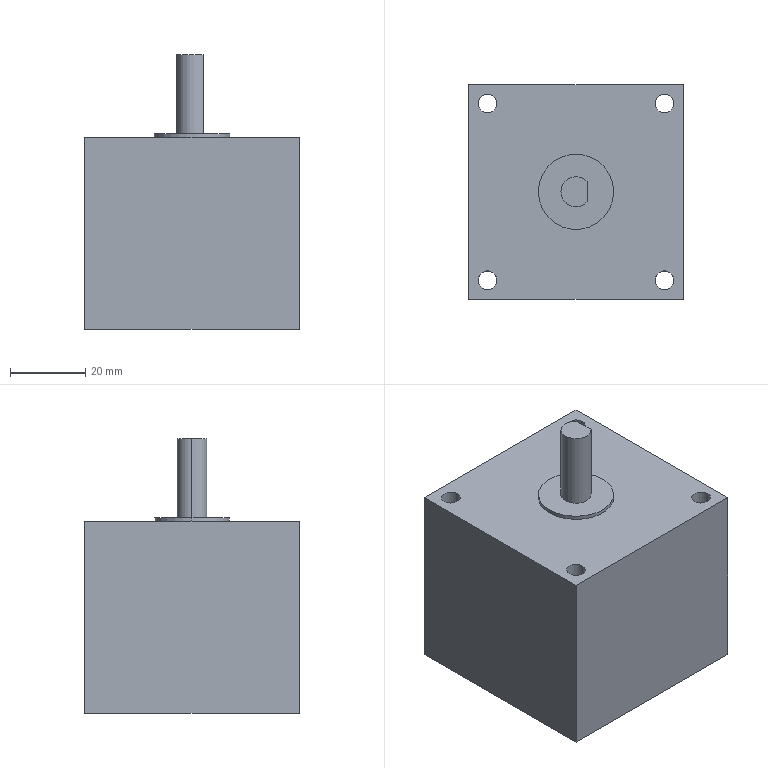Part | SolidWorks | features ICE 4, Extrusion 1 | 1 solid | 21 faces | box 57 x 57 x 73 mm | volume 162987 mm3 | cylinder 12 | plane 9 | commonest cylinder face diameters 5 x8 8 x2 20 x2
STEP:
#1=CARTESIAN_POINT('',(-4.,0.,73.));
#2=VERTEX_POINT('',#1);
#3=CARTESIAN_POINT('',(3.,-2.646,73.));
#4=VERTEX_POINT('',#3);
#5=CARTESIAN_POINT('',(0.,0.,73.));
#6=DIRECTION('',(0.,0.,1.));
#7=DIRECTION('',(1.,0.,0.));
#8=AXIS2_PLACEMENT_3D('',#5,#6,#7);
#9=CIRCLE('',#8,4.);
#10=EDGE_CURVE('',#2,#4,#9,.T.);
#11=ORIENTED_EDGE('',*,*,#10,.F.);
#12=CARTESIAN_POINT('',(-4.,0.,52.));
#13=VERTEX_POINT('',#12);
#14=CARTESIAN_POINT('',(-4.,0.,73.));
#15=DIRECTION('',(0.,0.,-1.));
#16=VECTOR('',#15,1000.);
#17=LINE('',#14,#16);
#18=EDGE_CURVE('',#2,#13,#17,.T.);
#19=ORIENTED_EDGE('',*,*,#18,.T.);
#20=CARTESIAN_POINT('',(3.,-2.646,52.));
#21=VERTEX_POINT('',#20);
#22=CARTESIAN_POINT('',(0.,0.,52.));
#23=DIRECTION('',(0.,0.,1.));
#24=DIRECTION('',(1.,0.,0.));
#25=AXIS2_PLACEMENT_3D('',#22,#23,#24);
#26=CIRCLE('',#25,4.);
#27=EDGE_CURVE('',#13,#21,#26,.T.);
#28=ORIENTED_EDGE('',*,*,#27,.T.);
#29=CARTESIAN_POINT('',(3.,-2.646,52.));
#30=DIRECTION('',(0.,0.,1.));
#31=VECTOR('',#30,1000.);
#32=LINE('',#29,#31);
#33=EDGE_CURVE('',#21,#4,#32,.T.);
#34=ORIENTED_EDGE('',*,*,#33,.T.);
#35=EDGE_LOOP('',(#11,#19,#28,#34));
#36=FACE_OUTER_BOUND('',#35,.T.);
#37=CARTESIAN_POINT('',(0.,0.,73.));
#38=DIRECTION('',(0.,0.,-1.));
#39=DIRECTION('',(-1.,0.,0.));
#40=AXIS2_PLACEMENT_3D('',#37,#38,#39);
#41=CYLINDRICAL_SURFACE('',#40,4.);
#42=ADVANCED_FACE('',(#36),#41,.T.);
#43=CARTESIAN_POINT('',(10.,0.,52.));
#44=VERTEX_POINT('',#43);
#45=CARTESIAN_POINT('',(-10.,0.,52.));
#46=VERTEX_POINT('',#45);
#47=CARTESIAN_POINT('',(0.,0.,52.));
#48=DIRECTION('',(0.,0.,1.));
#49=DIRECTION('',(1.,0.,0.));
#50=AXIS2_PLACEMENT_3D('',#47,#48,#49);
#51=CIRCLE('',#50,10.);
#52=EDGE_CURVE('',#44,#46,#51,.T.);
#53=ORIENTED_EDGE('',*,*,#52,.F.);
#54=CARTESIAN_POINT('',(10.,0.,51.));
#55=VERTEX_POINT('',#54);
#56=CARTESIAN_POINT('',(10.,0.,52.));
#57=DIRECTION('',(0.,0.,-1.));
#58=VECTOR('',#57,1000.);
#59=LINE('',#56,#58);
#60=EDGE_CURVE('',#44,#55,#59,.T.);
#61=ORIENTED_EDGE('',*,*,#60,.T.);
#62=CARTESIAN_POINT('',(-10.,0.,51.));
#63=VERTEX_POINT('',#62);
#64=CARTESIAN_POINT('',(0.,0.,51.));
#65=DIRECTION('',(0.,0.,1.));
#66=DIRECTION('',(1.,0.,0.));
#67=AXIS2_PLACEMENT_3D('',#64,#65,#66);
#68=CIRCLE('',#67,10.);
#69=EDGE_CURVE('',#55,#63,#68,.T.);
#70=ORIENTED_EDGE('',*,*,#69,.T.);
#71=CARTESIAN_POINT('',(-10.,0.,52.));
#72=DIRECTION('',(0.,0.,-1.));
#73=VECTOR('',#72,1000.);
#74=LINE('',#71,#73);
#75=EDGE_CURVE('',#46,#63,#74,.T.);
#76=ORIENTED_EDGE('',*,*,#75,.F.);
#77=EDGE_LOOP('',(#53,#61,#70,#76));
#78=FACE_OUTER_BOUND('',#77,.T.);
#79=CARTESIAN_POINT('',(0.,0.,52.));
#80=DIRECTION('',(0.,0.,-1.));
#81=DIRECTION('',(-1.,0.,0.));
#82=AXIS2_PLACEMENT_3D('',#79,#80,#81);
#83=CYLINDRICAL_SURFACE('',#82,10.);
#84=ADVANCED_FACE('',(#78),#83,.T.);
#85=CARTESIAN_POINT('',(-26.,-23.5,0.));
#86=VERTEX_POINT('',#85);
#87=CARTESIAN_POINT('',(-21.,-23.5,0.));
#88=VERTEX_POINT('',#87);
#89=CARTESIAN_POINT('',(-23.5,-23.5,0.));
#90=DIRECTION('',(0.,0.,1.));
#91=DIRECTION('',(1.,0.,0.));
#92=AXIS2_PLACEMENT_3D('',#89,#90,#91);
#93=CIRCLE('',#92,2.5);
#94=EDGE_CURVE('',#86,#88,#93,.T.);
#95=ORIENTED_EDGE('',*,*,#94,.F.);
#96=CARTESIAN_POINT('',(-26.,-23.5,51.));
#97=VERTEX_POINT('',#96);
#98=CARTESIAN_POINT('',(-26.,-23.5,-47.));
#99=DIRECTION('',(0.,0.,1.));
#100=VECTOR('',#99,1000.);
#101=LINE('',#98,#100);
#102=EDGE_CURVE('',#86,#97,#101,.T.);
#103=ORIENTED_EDGE('',*,*,#102,.T.);
#104=CARTESIAN_POINT('',(-21.,-23.5,51.));
#105=VERTEX_POINT('',#104);
#106=CARTESIAN_POINT('',(-23.5,-23.5,51.));
#107=DIRECTION('',(0.,0.,1.));
#108=DIRECTION('',(1.,0.,0.));
#109=AXIS2_PLACEMENT_3D('',#106,#107,#108);
#110=CIRCLE('',#109,2.5);
#111=EDGE_CURVE('',#97,#105,#110,.T.);
#112=ORIENTED_EDGE('',*,*,#111,.T.);
#113=CARTESIAN_POINT('',(-21.,-23.5,-47.));
#114=DIRECTION('',(0.,0.,1.));
#115=VECTOR('',#114,1000.);
#116=LINE('',#113,#115);
#117=EDGE_CURVE('',#88,#105,#116,.T.);
#118=ORIENTED_EDGE('',*,*,#117,.F.);
#119=EDGE_LOOP('',(#95,#103,#112,#118));
#120=FACE_OUTER_BOUND('',#119,.T.);
#121=CARTESIAN_POINT('',(-23.5,-23.5,-47.));
#122=DIRECTION('',(0.,0.,1.));
#123=DIRECTION('',(1.,0.,0.));
#124=AXIS2_PLACEMENT_3D('',#121,#122,#123);
#125=CYLINDRICAL_SURFACE('',#124,2.5);
#126=ADVANCED_FACE('',(#120),#125,.F.);
#127=CARTESIAN_POINT('',(21.,-23.5,0.));
#128=VERTEX_POINT('',#127);
#129=CARTESIAN_POINT('',(26.,-23.5,0.));
#130=VERTEX_POINT('',#129);
#131=CARTESIAN_POINT('',(23.5,-23.5,0.));
#132=DIRECTION('',(0.,0.,1.));
#133=DIRECTION('',(1.,0.,0.));
#134=AXIS2_PLACEMENT_3D('',#131,#132,#133);
#135=CIRCLE('',#134,2.5);
#136=EDGE_CURVE('',#128,#130,#135,.T.);
#137=ORIENTED_EDGE('',*,*,#136,.F.);
#138=CARTESIAN_POINT('',(21.,-23.5,51.));
#139=VERTEX_POINT('',#138);
#140=CARTESIAN_POINT('',(21.,-23.5,-47.));
#141=DIRECTION('',(0.,0.,1.));
#142=VECTOR('',#141,1000.);
#143=LINE('',#140,#142);
#144=EDGE_CURVE('',#128,#139,#143,.T.);
#145=ORIENTED_EDGE('',*,*,#144,.T.);
#146=CARTESIAN_POINT('',(26.,-23.5,51.));
#147=VERTEX_POINT('',#146);
#148=CARTESIAN_POINT('',(23.5,-23.5,51.));
#149=DIRECTION('',(0.,0.,1.));
#150=DIRECTION('',(1.,0.,0.));
#151=AXIS2_PLACEMENT_3D('',#148,#149,#150);
#152=CIRCLE('',#151,2.5);
#153=EDGE_CURVE('',#139,#147,#152,.T.);
#154=ORIENTED_EDGE('',*,*,#153,.T.);
#155=CARTESIAN_POINT('',(26.,-23.5,-47.));
#156=DIRECTION('',(0.,0.,1.));
#157=VECTOR('',#156,1000.);
#158=LINE('',#155,#157);
#159=EDGE_CURVE('',#130,#147,#158,.T.);
#160=ORIENTED_EDGE('',*,*,#159,.F.);
#161=EDGE_LOOP('',(#137,#145,#154,#160));
#162=FACE_OUTER_BOUND('',#161,.T.);
#163=CARTESIAN_POINT('',(23.5,-23.5,-47.));
#164=DIRECTION('',(0.,0.,1.));
#165=DIRECTION('',(1.,0.,0.));
#166=AXIS2_PLACEMENT_3D('',#163,#164,#165);
#167=CYLINDRICAL_SURFACE('',#166,2.5);
#168=ADVANCED_FACE('',(#162),#167,.F.);
#169=CARTESIAN_POINT('',(21.,23.5,0.));
#170=VERTEX_POINT('',#169);
#171=CARTESIAN_POINT('',(26.,23.5,0.));
#172=VERTEX_POINT('',#171);
#173=CARTESIAN_POINT('',(23.5,23.5,0.));
#174=DIRECTION('',(0.,0.,1.));
#175=DIRECTION('',(1.,0.,0.));
#176=AXIS2_PLACEMENT_3D('',#173,#174,#175);
#177=CIRCLE('',#176,2.5);
#178=EDGE_CURVE('',#170,#172,#177,.T.);
#179=ORIENTED_EDGE('',*,*,#178,.F.);
#180=CARTESIAN_POINT('',(21.,23.5,51.));
#181=VERTEX_POINT('',#180);
#182=CARTESIAN_POINT('',(21.,23.5,-47.));
#183=DIRECTION('',(0.,0.,1.));
#184=VECTOR('',#183,1000.);
#185=LINE('',#182,#184);
#186=EDGE_CURVE('',#170,#181,#185,.T.);
#187=ORIENTED_EDGE('',*,*,#186,.T.);
#188=CARTESIAN_POINT('',(26.,23.5,51.));
#189=VERTEX_POINT('',#188);
#190=CARTESIAN_POINT('',(23.5,23.5,51.));
#191=DIRECTION('',(0.,0.,1.));
#192=DIRECTION('',(1.,0.,0.));
#193=AXIS2_PLACEMENT_3D('',#190,#191,#192);
#194=CIRCLE('',#193,2.5);
#195=EDGE_CURVE('',#181,#189,#194,.T.);
#196=ORIENTED_EDGE('',*,*,#195,.T.);
#197=CARTESIAN_POINT('',(26.,23.5,-47.));
#198=DIRECTION('',(0.,0.,1.));
#199=VECTOR('',#198,1000.);
#200=LINE('',#197,#199);
#201=EDGE_CURVE('',#172,#189,#200,.T.);
#202=ORIENTED_EDGE('',*,*,#201,.F.);
#203=EDGE_LOOP('',(#179,#187,#196,#202));
#204=FACE_OUTER_BOUND('',#203,.T.);
#205=CARTESIAN_POINT('',(23.5,23.5,-47.));
#206=DIRECTION('',(0.,0.,1.));
#207=DIRECTION('',(1.,0.,0.));
#208=AXIS2_PLACEMENT_3D('',#205,#206,#207);
#209=CYLINDRICAL_SURFACE('',#208,2.5);
#210=ADVANCED_FACE('',(#204),#209,.F.);
#211=CARTESIAN_POINT('',(-26.,23.5,0.));
#212=VERTEX_POINT('',#211);
#213=CARTESIAN_POINT('',(-21.,23.5,0.));
#214=VERTEX_POINT('',#213);
#215=CARTESIAN_POINT('',(-23.5,23.5,0.));
#216=DIRECTION('',(0.,0.,1.));
#217=DIRECTION('',(1.,0.,0.));
#218=AXIS2_PLACEMENT_3D('',#215,#216,#217);
#219=CIRCLE('',#218,2.5);
#220=EDGE_CURVE('',#212,#214,#219,.T.);
#221=ORIENTED_EDGE('',*,*,#220,.F.);
#222=CARTESIAN_POINT('',(-26.,23.5,51.));
#223=VERTEX_POINT('',#222);
#224=CARTESIAN_POINT('',(-26.,23.5,-47.));
#225=DIRECTION('',(0.,0.,1.));
#226=VECTOR('',#225,1000.);
#227=LINE('',#224,#226);
#228=EDGE_CURVE('',#212,#223,#227,.T.);
#229=ORIENTED_EDGE('',*,*,#228,.T.);
#230=CARTESIAN_POINT('',(-21.,23.5,51.));
#231=VERTEX_POINT('',#230);
#232=CARTESIAN_POINT('',(-23.5,23.5,51.));
#233=DIRECTION('',(0.,0.,1.));
#234=DIRECTION('',(1.,0.,0.));
#235=AXIS2_PLACEMENT_3D('',#232,#233,#234);
#236=CIRCLE('',#235,2.5);
#237=EDGE_CURVE('',#223,#231,#236,.T.);
#238=ORIENTED_EDGE('',*,*,#237,.T.);
#239=CARTESIAN_POINT('',(-21.,23.5,-47.));
#240=DIRECTION('',(0.,0.,1.));
#241=VECTOR('',#240,1000.);
#242=LINE('',#239,#241);
#243=EDGE_CURVE('',#214,#231,#242,.T.);
#244=ORIENTED_EDGE('',*,*,#243,.F.);
#245=EDGE_LOOP('',(#221,#229,#238,#244));
#246=FACE_OUTER_BOUND('',#245,.T.);
#247=CARTESIAN_POINT('',(-23.5,23.5,-47.));
#248=DIRECTION('',(0.,0.,1.));
#249=DIRECTION('',(1.,0.,0.));
#250=AXIS2_PLACEMENT_3D('',#247,#248,#249);
#251=CYLINDRICAL_SURFACE('',#250,2.5);
#252=ADVANCED_FACE('',(#246),#251,.F.);
#253=CARTESIAN_POINT('',(-28.5,28.5,0.));
#254=VERTEX_POINT('',#253);
#255=CARTESIAN_POINT('',(-28.5,-28.5,0.));
#256=VERTEX_POINT('',#255);
#257=CARTESIAN_POINT('',(-28.5,-28.5,0.));
#258=DIRECTION('',(0.,-1.,0.));
#259=VECTOR('',#258,1000.);
#260=LINE('',#257,#259);
#261=EDGE_CURVE('',#254,#256,#260,.T.);
#262=ORIENTED_EDGE('',*,*,#261,.T.);
#263=CARTESIAN_POINT('',(-28.5,-28.5,51.));
#264=VERTEX_POINT('',#263);
#265=CARTESIAN_POINT('',(-28.5,-28.5,51.));
#266=DIRECTION('',(0.,0.,-1.));
#267=VECTOR('',#266,1000.);
#268=LINE('',#265,#267);
#269=EDGE_CURVE('',#264,#256,#268,.T.);
#270=ORIENTED_EDGE('',*,*,#269,.F.);
#271=CARTESIAN_POINT('',(-28.5,28.5,51.));
#272=VERTEX_POINT('',#271);
#273=CARTESIAN_POINT('',(-28.5,-28.5,51.));
#274=DIRECTION('',(0.,-1.,0.));
#275=VECTOR('',#274,1000.);
#276=LINE('',#273,#275);
#277=EDGE_CURVE('',#272,#264,#276,.T.);
#278=ORIENTED_EDGE('',*,*,#277,.F.);
#279=CARTESIAN_POINT('',(-28.5,28.5,51.));
#280=DIRECTION('',(0.,0.,-1.));
#281=VECTOR('',#280,1000.);
#282=LINE('',#279,#281);
#283=EDGE_CURVE('',#272,#254,#282,.T.);
#284=ORIENTED_EDGE('',*,*,#283,.T.);
#285=EDGE_LOOP('',(#262,#270,#278,#284));
#286=FACE_OUTER_BOUND('',#285,.T.);
#287=CARTESIAN_POINT('',(-28.5,-28.5,51.));
#288=DIRECTION('',(1.,0.,0.));
#289=DIRECTION('',(0.,0.,-1.));
#290=AXIS2_PLACEMENT_3D('',#287,#288,#289);
#291=PLANE('',#290);
#292=ADVANCED_FACE('',(#286),#291,.F.);
#293=CARTESIAN_POINT('',(28.5,-28.5,0.));
#294=VERTEX_POINT('',#293);
#295=CARTESIAN_POINT('',(28.5,-28.5,0.));
#296=DIRECTION('',(1.,0.,0.));
#297=VECTOR('',#296,1000.);
#298=LINE('',#295,#297);
#299=EDGE_CURVE('',#256,#294,#298,.T.);
#300=ORIENTED_EDGE('',*,*,#299,.T.);
#301=CARTESIAN_POINT('',(28.5,-28.5,51.));
#302=VERTEX_POINT('',#301);
#303=CARTESIAN_POINT('',(28.5,-28.5,51.));
#304=DIRECTION('',(0.,0.,-1.));
#305=VECTOR('',#304,1000.);
#306=LINE('',#303,#305);
#307=EDGE_CURVE('',#302,#294,#306,.T.);
#308=ORIENTED_EDGE('',*,*,#307,.F.);
#309=CARTESIAN_POINT('',(28.5,-28.5,51.));
#310=DIRECTION('',(1.,0.,0.));
#311=VECTOR('',#310,1000.);
#312=LINE('',#309,#311);
#313=EDGE_CURVE('',#264,#302,#312,.T.);
#314=ORIENTED_EDGE('',*,*,#313,.F.);
#315=ORIENTED_EDGE('',*,*,#269,.T.);
#316=EDGE_LOOP('',(#300,#308,#314,#315));
#317=FACE_OUTER_BOUND('',#316,.T.);
#318=CARTESIAN_POINT('',(28.5,-28.5,51.));
#319=DIRECTION('',(0.,1.,0.));
#320=DIRECTION('',(-1.,0.,0.));
#321=AXIS2_PLACEMENT_3D('',#318,#319,#320);
#322=PLANE('',#321);
#323=ADVANCED_FACE('',(#317),#322,.F.);
#324=CARTESIAN_POINT('',(28.5,28.5,0.));
#325=VERTEX_POINT('',#324);
#326=CARTESIAN_POINT('',(28.5,-28.5,0.));
#327=DIRECTION('',(0.,1.,0.));
#328=VECTOR('',#327,1000.);
#329=LINE('',#326,#328);
#330=EDGE_CURVE('',#294,#325,#329,.T.);
#331=ORIENTED_EDGE('',*,*,#330,.T.);
#332=CARTESIAN_POINT('',(28.5,28.5,51.));
#333=VERTEX_POINT('',#332);
#334=CARTESIAN_POINT('',(28.5,28.5,51.));
#335=DIRECTION('',(0.,0.,-1.));
#336=VECTOR('',#335,1000.);
#337=LINE('',#334,#336);
#338=EDGE_CURVE('',#333,#325,#337,.T.);
#339=ORIENTED_EDGE('',*,*,#338,.F.);
#340=CARTESIAN_POINT('',(28.5,-28.5,51.));
#341=DIRECTION('',(0.,1.,0.));
#342=VECTOR('',#341,1000.);
#343=LINE('',#340,#342);
#344=EDGE_CURVE('',#302,#333,#343,.T.);
#345=ORIENTED_EDGE('',*,*,#344,.F.);
#346=ORIENTED_EDGE('',*,*,#307,.T.);
#347=EDGE_LOOP('',(#331,#339,#345,#346));
#348=FACE_OUTER_BOUND('',#347,.T.);
#349=CARTESIAN_POINT('',(28.5,-28.5,51.));
#350=DIRECTION('',(-1.,0.,0.));
#351=DIRECTION('',(0.,0.,1.));
#352=AXIS2_PLACEMENT_3D('',#349,#350,#351);
#353=PLANE('',#352);
#354=ADVANCED_FACE('',(#348),#353,.F.);
#355=CARTESIAN_POINT('',(28.5,28.5,0.));
#356=DIRECTION('',(-1.,0.,0.));
#357=VECTOR('',#356,1000.);
#358=LINE('',#355,#357);
#359=EDGE_CURVE('',#325,#254,#358,.T.);
#360=ORIENTED_EDGE('',*,*,#359,.T.);
#361=ORIENTED_EDGE('',*,*,#283,.F.);
#362=CARTESIAN_POINT('',(28.5,28.5,51.));
#363=DIRECTION('',(-1.,0.,0.));
#364=VECTOR('',#363,1000.);
#365=LINE('',#362,#364);
#366=EDGE_CURVE('',#333,#272,#365,.T.);
#367=ORIENTED_EDGE('',*,*,#366,.F.);
#368=ORIENTED_EDGE('',*,*,#338,.T.);
#369=EDGE_LOOP('',(#360,#361,#367,#368));
#370=FACE_OUTER_BOUND('',#369,.T.);
#371=CARTESIAN_POINT('',(28.5,28.5,51.));
#372=DIRECTION('',(0.,-1.,0.));
#373=DIRECTION('',(1.,0.,0.));
#374=AXIS2_PLACEMENT_3D('',#371,#372,#373);
#375=PLANE('',#374);
#376=ADVANCED_FACE('',(#370),#375,.F.);
#377=CARTESIAN_POINT('',(0.,0.,51.));
#378=DIRECTION('',(0.,0.,1.));
#379=DIRECTION('',(1.,0.,0.));
#380=AXIS2_PLACEMENT_3D('',#377,#378,#379);
#381=CIRCLE('',#380,10.);
#382=EDGE_CURVE('',#63,#55,#381,.T.);
#383=ORIENTED_EDGE('',*,*,#382,.F.);
#384=ORIENTED_EDGE('',*,*,#69,.F.);
#385=EDGE_LOOP('',(#383,#384));
#386=FACE_BOUND('',#385,.T.);
#387=CARTESIAN_POINT('',(-23.5,-23.5,51.));
#388=DIRECTION('',(0.,0.,1.));
#389=DIRECTION('',(1.,0.,0.));
#390=AXIS2_PLACEMENT_3D('',#387,#388,#389);
#391=CIRCLE('',#390,2.5);
#392=EDGE_CURVE('',#105,#97,#391,.T.);
#393=ORIENTED_EDGE('',*,*,#392,.F.);
#394=ORIENTED_EDGE('',*,*,#111,.F.);
#395=EDGE_LOOP('',(#393,#394));
#396=FACE_BOUND('',#395,.T.);
#397=CARTESIAN_POINT('',(23.5,-23.5,51.));
#398=DIRECTION('',(0.,0.,1.));
#399=DIRECTION('',(1.,0.,0.));
#400=AXIS2_PLACEMENT_3D('',#397,#398,#399);
#401=CIRCLE('',#400,2.5);
#402=EDGE_CURVE('',#147,#139,#401,.T.);
#403=ORIENTED_EDGE('',*,*,#402,.F.);
#404=ORIENTED_EDGE('',*,*,#153,.F.);
#405=EDGE_LOOP('',(#403,#404));
#406=FACE_BOUND('',#405,.T.);
#407=CARTESIAN_POINT('',(23.5,23.5,51.));
#408=DIRECTION('',(0.,0.,1.));
#409=DIRECTION('',(1.,0.,0.));
#410=AXIS2_PLACEMENT_3D('',#407,#408,#409);
#411=CIRCLE('',#410,2.5);
#412=EDGE_CURVE('',#189,#181,#411,.T.);
#413=ORIENTED_EDGE('',*,*,#412,.F.);
#414=ORIENTED_EDGE('',*,*,#195,.F.);
#415=EDGE_LOOP('',(#413,#414));
#416=FACE_BOUND('',#415,.T.);
#417=CARTESIAN_POINT('',(-23.5,23.5,51.));
#418=DIRECTION('',(0.,0.,1.));
#419=DIRECTION('',(1.,0.,0.));
#420=AXIS2_PLACEMENT_3D('',#417,#418,#419);
#421=CIRCLE('',#420,2.5);
#422=EDGE_CURVE('',#231,#223,#421,.T.);
#423=ORIENTED_EDGE('',*,*,#422,.F.);
#424=ORIENTED_EDGE('',*,*,#237,.F.);
#425=EDGE_LOOP('',(#423,#424));
#426=FACE_BOUND('',#425,.T.);
#427=ORIENTED_EDGE('',*,*,#277,.T.);
#428=ORIENTED_EDGE('',*,*,#313,.T.);
#429=ORIENTED_EDGE('',*,*,#344,.T.);
#430=ORIENTED_EDGE('',*,*,#366,.T.);
#431=EDGE_LOOP('',(#427,#428,#429,#430));
#432=FACE_OUTER_BOUND('',#431,.T.);
#433=CARTESIAN_POINT('',(0.,0.,51.));
#434=DIRECTION('',(0.,0.,1.));
#435=DIRECTION('',(1.,0.,0.));
#436=AXIS2_PLACEMENT_3D('',#433,#434,#435);
#437=PLANE('',#436);
#438=ADVANCED_FACE('',(#386,#396,#406,#416,#426,#432),#437,.T.);
#439=CARTESIAN_POINT('',(-23.5,-23.5,0.));
#440=DIRECTION('',(0.,0.,1.));
#441=DIRECTION('',(1.,0.,0.));
#442=AXIS2_PLACEMENT_3D('',#439,#440,#441);
#443=CIRCLE('',#442,2.5);
#444=EDGE_CURVE('',#88,#86,#443,.T.);
#445=ORIENTED_EDGE('',*,*,#444,.T.);
#446=ORIENTED_EDGE('',*,*,#94,.T.);
#447=EDGE_LOOP('',(#445,#446));
#448=FACE_BOUND('',#447,.T.);
#449=CARTESIAN_POINT('',(23.5,-23.5,0.));
#450=DIRECTION('',(0.,0.,1.));
#451=DIRECTION('',(1.,0.,0.));
#452=AXIS2_PLACEMENT_3D('',#449,#450,#451);
#453=CIRCLE('',#452,2.5);
#454=EDGE_CURVE('',#130,#128,#453,.T.);
#455=ORIENTED_EDGE('',*,*,#454,.T.);
#456=ORIENTED_EDGE('',*,*,#136,.T.);
#457=EDGE_LOOP('',(#455,#456));
#458=FACE_BOUND('',#457,.T.);
#459=CARTESIAN_POINT('',(23.5,23.5,0.));
#460=DIRECTION('',(0.,0.,1.));
#461=DIRECTION('',(1.,0.,0.));
#462=AXIS2_PLACEMENT_3D('',#459,#460,#461);
#463=CIRCLE('',#462,2.5);
#464=EDGE_CURVE('',#172,#170,#463,.T.);
#465=ORIENTED_EDGE('',*,*,#464,.T.);
#466=ORIENTED_EDGE('',*,*,#178,.T.);
#467=EDGE_LOOP('',(#465,#466));
#468=FACE_BOUND('',#467,.T.);
#469=CARTESIAN_POINT('',(-23.5,23.5,0.));
#470=DIRECTION('',(0.,0.,1.));
#471=DIRECTION('',(1.,0.,0.));
#472=AXIS2_PLACEMENT_3D('',#469,#470,#471);
#473=CIRCLE('',#472,2.5);
#474=EDGE_CURVE('',#214,#212,#473,.T.);
#475=ORIENTED_EDGE('',*,*,#474,.T.);
#476=ORIENTED_EDGE('',*,*,#220,.T.);
#477=EDGE_LOOP('',(#475,#476));
#478=FACE_BOUND('',#477,.T.);
#479=ORIENTED_EDGE('',*,*,#261,.F.);
#480=ORIENTED_EDGE('',*,*,#359,.F.);
#481=ORIENTED_EDGE('',*,*,#330,.F.);
#482=ORIENTED_EDGE('',*,*,#299,.F.);
#483=EDGE_LOOP('',(#479,#480,#481,#482));
#484=FACE_OUTER_BOUND('',#483,.T.);
#485=CARTESIAN_POINT('',(0.,0.,0.));
#486=DIRECTION('',(0.,0.,1.));
#487=DIRECTION('',(1.,0.,0.));
#488=AXIS2_PLACEMENT_3D('',#485,#486,#487);
#489=PLANE('',#488);
#490=ADVANCED_FACE('',(#448,#458,#468,#478,#484),#489,.F.);
#491=ORIENTED_EDGE('',*,*,#228,.F.);
#492=ORIENTED_EDGE('',*,*,#474,.F.);
#493=ORIENTED_EDGE('',*,*,#243,.T.);
#494=ORIENTED_EDGE('',*,*,#422,.T.);
#495=EDGE_LOOP('',(#491,#492,#493,#494));
#496=FACE_OUTER_BOUND('',#495,.T.);
#497=CARTESIAN_POINT('',(-23.5,23.5,-47.));
#498=DIRECTION('',(0.,0.,1.));
#499=DIRECTION('',(1.,0.,0.));
#500=AXIS2_PLACEMENT_3D('',#497,#498,#499);
#501=CYLINDRICAL_SURFACE('',#500,2.5);
#502=ADVANCED_FACE('',(#496),#501,.F.);
#503=ORIENTED_EDGE('',*,*,#186,.F.);
#504=ORIENTED_EDGE('',*,*,#464,.F.);
#505=ORIENTED_EDGE('',*,*,#201,.T.);
#506=ORIENTED_EDGE('',*,*,#412,.T.);
#507=EDGE_LOOP('',(#503,#504,#505,#506));
#508=FACE_OUTER_BOUND('',#507,.T.);
#509=CARTESIAN_POINT('',(23.5,23.5,-47.));
#510=DIRECTION('',(0.,0.,1.));
#511=DIRECTION('',(1.,0.,0.));
#512=AXIS2_PLACEMENT_3D('',#509,#510,#511);
#513=CYLINDRICAL_SURFACE('',#512,2.5);
#514=ADVANCED_FACE('',(#508),#513,.F.);
#515=ORIENTED_EDGE('',*,*,#144,.F.);
#516=ORIENTED_EDGE('',*,*,#454,.F.);
#517=ORIENTED_EDGE('',*,*,#159,.T.);
#518=ORIENTED_EDGE('',*,*,#402,.T.);
#519=EDGE_LOOP('',(#515,#516,#517,#518));
#520=FACE_OUTER_BOUND('',#519,.T.);
#521=CARTESIAN_POINT('',(23.5,-23.5,-47.));
#522=DIRECTION('',(0.,0.,1.));
#523=DIRECTION('',(1.,0.,0.));
#524=AXIS2_PLACEMENT_3D('',#521,#522,#523);
#525=CYLINDRICAL_SURFACE('',#524,2.5);
#526=ADVANCED_FACE('',(#520),#525,.F.);
#527=ORIENTED_EDGE('',*,*,#102,.F.);
#528=ORIENTED_EDGE('',*,*,#444,.F.);
#529=ORIENTED_EDGE('',*,*,#117,.T.);
#530=ORIENTED_EDGE('',*,*,#392,.T.);
#531=EDGE_LOOP('',(#527,#528,#529,#530));
#532=FACE_OUTER_BOUND('',#531,.T.);
#533=CARTESIAN_POINT('',(-23.5,-23.5,-47.));
#534=DIRECTION('',(0.,0.,1.));
#535=DIRECTION('',(1.,0.,0.));
#536=AXIS2_PLACEMENT_3D('',#533,#534,#535);
#537=CYLINDRICAL_SURFACE('',#536,2.5);
#538=ADVANCED_FACE('',(#532),#537,.F.);
#539=ORIENTED_EDGE('',*,*,#60,.F.);
#540=CARTESIAN_POINT('',(0.,0.,52.));
#541=DIRECTION('',(0.,0.,1.));
#542=DIRECTION('',(1.,0.,0.));
#543=AXIS2_PLACEMENT_3D('',#540,#541,#542);
#544=CIRCLE('',#543,10.);
#545=EDGE_CURVE('',#46,#44,#544,.T.);
#546=ORIENTED_EDGE('',*,*,#545,.F.);
#547=ORIENTED_EDGE('',*,*,#75,.T.);
#548=ORIENTED_EDGE('',*,*,#382,.T.);
#549=EDGE_LOOP('',(#539,#546,#547,#548));
#550=FACE_OUTER_BOUND('',#549,.T.);
#551=CARTESIAN_POINT('',(0.,0.,52.));
#552=DIRECTION('',(0.,0.,-1.));
#553=DIRECTION('',(-1.,0.,0.));
#554=AXIS2_PLACEMENT_3D('',#551,#552,#553);
#555=CYLINDRICAL_SURFACE('',#554,10.);
#556=ADVANCED_FACE('',(#550),#555,.T.);
#557=CARTESIAN_POINT('',(3.,2.646,52.));
#558=VERTEX_POINT('',#557);
#559=CARTESIAN_POINT('',(0.,0.,52.));
#560=DIRECTION('',(0.,0.,1.));
#561=DIRECTION('',(1.,0.,0.));
#562=AXIS2_PLACEMENT_3D('',#559,#560,#561);
#563=CIRCLE('',#562,4.);
#564=EDGE_CURVE('',#558,#13,#563,.T.);
#565=ORIENTED_EDGE('',*,*,#564,.F.);
#566=CARTESIAN_POINT('',(3.,0.,52.));
#567=DIRECTION('',(0.,-1.,0.));
#568=VECTOR('',#567,1000.);
#569=LINE('',#566,#568);
#570=EDGE_CURVE('',#558,#21,#569,.T.);
#571=ORIENTED_EDGE('',*,*,#570,.T.);
#572=ORIENTED_EDGE('',*,*,#27,.F.);
#573=EDGE_LOOP('',(#565,#571,#572));
#574=FACE_BOUND('',#573,.T.);
#575=ORIENTED_EDGE('',*,*,#545,.T.);
#576=ORIENTED_EDGE('',*,*,#52,.T.);
#577=EDGE_LOOP('',(#575,#576));
#578=FACE_OUTER_BOUND('',#577,.T.);
#579=CARTESIAN_POINT('',(0.,0.,52.));
#580=DIRECTION('',(0.,0.,1.));
#581=DIRECTION('',(1.,0.,0.));
#582=AXIS2_PLACEMENT_3D('',#579,#580,#581);
#583=PLANE('',#582);
#584=ADVANCED_FACE('',(#574,#578),#583,.T.);
#585=ORIENTED_EDGE('',*,*,#18,.F.);
#586=CARTESIAN_POINT('',(3.,2.646,73.));
#587=VERTEX_POINT('',#586);
#588=CARTESIAN_POINT('',(0.,0.,73.));
#589=DIRECTION('',(0.,0.,1.));
#590=DIRECTION('',(1.,0.,0.));
#591=AXIS2_PLACEMENT_3D('',#588,#589,#590);
#592=CIRCLE('',#591,4.);
#593=EDGE_CURVE('',#587,#2,#592,.T.);
#594=ORIENTED_EDGE('',*,*,#593,.F.);
#595=CARTESIAN_POINT('',(3.,2.646,52.));
#596=DIRECTION('',(0.,0.,1.));
#597=VECTOR('',#596,1000.);
#598=LINE('',#595,#597);
#599=EDGE_CURVE('',#558,#587,#598,.T.);
#600=ORIENTED_EDGE('',*,*,#599,.F.);
#601=ORIENTED_EDGE('',*,*,#564,.T.);
#602=EDGE_LOOP('',(#585,#594,#600,#601));
#603=FACE_OUTER_BOUND('',#602,.T.);
#604=CARTESIAN_POINT('',(0.,0.,73.));
#605=DIRECTION('',(0.,0.,-1.));
#606=DIRECTION('',(-1.,0.,0.));
#607=AXIS2_PLACEMENT_3D('',#604,#605,#606);
#608=CYLINDRICAL_SURFACE('',#607,4.);
#609=ADVANCED_FACE('',(#603),#608,.T.);
#610=CARTESIAN_POINT('',(3.,0.,73.));
#611=DIRECTION('',(0.,-1.,0.));
#612=VECTOR('',#611,1000.);
#613=LINE('',#610,#612);
#614=EDGE_CURVE('',#587,#4,#613,.T.);
#615=ORIENTED_EDGE('',*,*,#614,.F.);
#616=ORIENTED_EDGE('',*,*,#593,.T.);
#617=ORIENTED_EDGE('',*,*,#10,.T.);
#618=EDGE_LOOP('',(#615,#616,#617));
#619=FACE_OUTER_BOUND('',#618,.T.);
#620=CARTESIAN_POINT('',(0.,0.,73.));
#621=DIRECTION('',(0.,0.,1.));
#622=DIRECTION('',(1.,0.,0.));
#623=AXIS2_PLACEMENT_3D('',#620,#621,#622);
#624=PLANE('',#623);
#625=ADVANCED_FACE('',(#619),#624,.T.);
#626=ORIENTED_EDGE('',*,*,#614,.T.);
#627=ORIENTED_EDGE('',*,*,#33,.F.);
#628=ORIENTED_EDGE('',*,*,#570,.F.);
#629=ORIENTED_EDGE('',*,*,#599,.T.);
#630=EDGE_LOOP('',(#626,#627,#628,#629));
#631=FACE_OUTER_BOUND('',#630,.T.);
#632=CARTESIAN_POINT('',(3.,0.,52.));
#633=DIRECTION('',(-1.,0.,0.));
#634=DIRECTION('',(0.,0.,1.));
#635=AXIS2_PLACEMENT_3D('',#632,#633,#634);
#636=PLANE('',#635);
#637=ADVANCED_FACE('',(#631),#636,.F.);
#638=CLOSED_SHELL('',(#42,#84,#126,#168,#210,#252,#292,#323,#354,#376,#438,#490,#502,#514,#526,#538,#556,#584,#609,#625,#637));
#639=MANIFOLD_SOLID_BREP('',#638);
#640=CARTESIAN_POINT('',(0.,0.,0.));
#641=DIRECTION('',(0.,0.,1.));
#642=DIRECTION('',(1.,0.,0.));
#643=AXIS2_PLACEMENT_3D('',#640,#641,#642);
#644=(LENGTH_UNIT()NAMED_UNIT(*)SI_UNIT(.MILLI.,.METRE.));
#645=UNCERTAINTY_MEASURE_WITH_UNIT(LENGTH_MEASURE(0.00001),#644,'','');
#646=(NAMED_UNIT(*)PLANE_ANGLE_UNIT()SI_UNIT($,.RADIAN.));
#647=(NAMED_UNIT(*)SI_UNIT($,.STERADIAN.)SOLID_ANGLE_UNIT());
#648=(GEOMETRIC_REPRESENTATION_CONTEXT(3)GLOBAL_UNCERTAINTY_ASSIGNED_CONTEXT((#645))GLOBAL_UNIT_ASSIGNED_CONTEXT((#644,#646,#647))REPRESENTATION_CONTEXT('',''));
#649=ADVANCED_BREP_SHAPE_REPRESENTATION('',(#639,#643),#648);